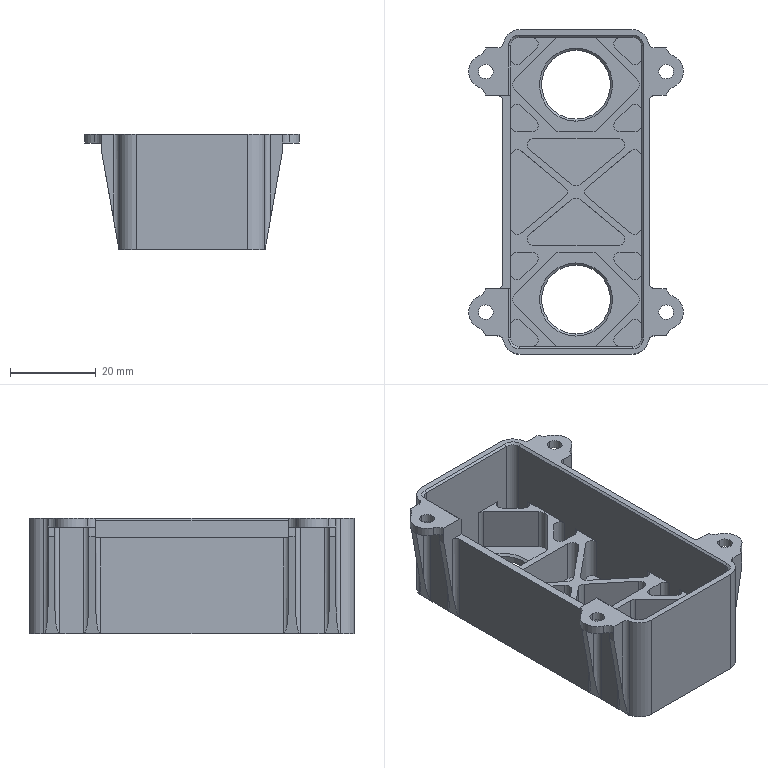NC program | NX | posted with a generic post | part box 50 x 75.58 x 26.8 mm
Lines 2647 to 3615 of 35818:
(CAVITY_MILL_COPY_COPY , TOOL : D4)
N5268 T11 M6
N5270 G54
N5272 G17 G0 G90 X-12.812 Y-30.466 S9500 M3
N5274 G43 Z30. H11
N5276 Z0.912
N5278 G94 G1 Z-0.088 F1000.
N5280 X-13.112 Y-30.639
N5282 G3 X-13.612 Y-31.505 R1.
N5284 G1 Y-33.99 F1400.
N5286 G3 X-13.2 Y-34.402 R0.412
N5288 G1 X-10.715
N5290 G3 X-9.849 Y-33.902 R1.
N5292 G1 X-9.676 Y-33.602
N5294 Z0.912
N5296 G0 X-12.413 Y-30.067 Z0.513
N5298 G1 Z-0.487 F1000.
N5300 X-12.713 Y-30.24
N5302 G3 X-13.213 Y-31.106 R1.
N5304 G1 Y-33.99 F1400.
N5306 X-13.214 Y-34.004
N5308 X-13.2 Y-34.003
N5310 X-10.316
N5312 G3 X-9.45 Y-33.503 R1.
N5314 G1 X-9.277 Y-33.203
N5316 Z0.513
N5318 G0 X-12.4 Y-30.054 Z0.114
N5320 G1 Z-0.886 F1000.
N5322 X-12.7 Y-30.227
N5324 G3 X-13.2 Y-31.093 R1.
N5326 G1 Y-33.99 F1400.
N5328 X-10.303
N5330 G3 X-9.437 Y-33.49 R1.
N5332 G1 X-9.264 Y-33.19
N5334 Z0.114
N5336 G0 X-12.4 Y-30.054 Z-0.284
N5338 G1 Z-1.284 F1000.
N5340 X-12.7 Y-30.227
N5342 G3 X-13.2 Y-31.093 R1.
N5344 G1 Y-33.99 F1400.
N5346 X-10.303
N5348 G3 X-9.437 Y-33.49 R1.
N5350 G1 X-9.264 Y-33.19
N5352 Z-0.284
N5354 G0 X-12.4 Y-30.054 Z-0.683
N5356 G1 Z-1.683 F1000.
N5358 X-12.7 Y-30.227
N5360 G3 X-13.2 Y-31.093 R1.
N5362 G1 Y-33.99 F1400.
N5364 X-10.303
N5366 G3 X-9.437 Y-33.49 R1.
N5368 G1 X-9.264 Y-33.19
N5370 Z-0.683
N5372 G0 X-12.4 Y-30.054 Z-1.082
N5374 G1 Z-2.082 F1000.
N5376 X-12.7 Y-30.227
N5378 G3 X-13.2 Y-31.093 R1.
N5380 G1 Y-33.99 F1400.
N5382 X-10.303
N5384 G3 X-9.437 Y-33.49 R1.
N5386 G1 X-9.264 Y-33.19
N5388 Z-1.082
N5390 G0 X-12.4 Y-30.054 Z-1.48
N5392 G1 Z-2.48 F1000.
N5394 X-12.7 Y-30.227
N5396 G3 X-13.2 Y-31.093 R1.
N5398 G1 Y-33.99 F1400.
N5400 X-10.303
N5402 G3 X-9.437 Y-33.49 R1.
N5404 G1 X-9.264 Y-33.19
N5406 Z-1.48
N5408 G0 X-12.4 Y-30.054 Z-1.879
N5410 G1 Z-2.879 F1000.
N5412 X-12.7 Y-30.227
N5414 G3 X-13.2 Y-31.093 R1.
N5416 G1 Y-33.99 F1400.
N5418 X-10.303
N5420 G3 X-9.437 Y-33.49 R1.
N5422 G1 X-9.264 Y-33.19
N5424 Z-1.879
N5426 G0 X-12.4 Y-30.054 Z-2.278
N5428 G1 Z-3.278 F1000.
N5430 X-12.7 Y-30.227
N5432 G3 X-13.2 Y-31.093 R1.
N5434 G1 Y-33.99 F1400.
N5436 X-10.303
N5438 G3 X-9.437 Y-33.49 R1.
N5440 G1 X-9.264 Y-33.19
N5442 Z-2.278
N5444 G0 X-12.4 Y-30.054 Z-2.676
N5446 G1 Z-3.676 F1000.
N5448 X-12.7 Y-30.227
N5450 G3 X-13.2 Y-31.093 R1.
N5452 G1 Y-33.99 F1400.
N5454 X-10.303
N5456 G3 X-9.437 Y-33.49 R1.
N5458 G1 X-9.264 Y-33.19
N5460 Z-2.676
N5462 G0 X-12.4 Y-30.054 Z-3.075
N5464 G1 Z-4.075 F1000.
N5466 X-12.7 Y-30.227
N5468 G3 X-13.2 Y-31.093 R1.
N5470 G1 Y-33.99 F1400.
N5472 X-10.303
N5474 G3 X-9.437 Y-33.49 R1.
N5476 G1 X-9.264 Y-33.19
N5478 Z-3.075
N5480 G0 X-12.4 Y-30.054 Z-3.474
N5482 G1 Z-4.474 F1000.
N5484 X-12.7 Y-30.227
N5486 G3 X-13.2 Y-31.093 R1.
N5488 G1 Y-33.99 F1400.
N5490 X-10.303
N5492 G3 X-9.437 Y-33.49 R1.
N5494 G1 X-9.264 Y-33.19
N5496 Z-3.474
N5498 G0 X-12.4 Y-30.054 Z-3.872
N5500 G1 Z-4.872 F1000.
N5502 X-12.7 Y-30.227
N5504 G3 X-13.2 Y-31.093 R1.
N5506 G1 Y-33.99 F1400.
N5508 X-10.303
N5510 G3 X-9.437 Y-33.49 R1.
N5512 G1 X-9.264 Y-33.19
N5514 Z-3.872
N5516 G0 X-12.4 Y-30.054 Z-4.271
N5518 G1 Z-5.271 F1000.
N5520 X-12.7 Y-30.227
N5522 G3 X-13.2 Y-31.093 R1.
N5524 G1 Y-33.99 F1400.
N5526 X-10.303
N5528 G3 X-9.437 Y-33.49 R1.
N5530 G1 X-9.264 Y-33.19
N5532 Z-4.271
N5534 G0 X-12.4 Y-30.054 Z-4.67
N5536 G1 Z-5.67 F1000.
N5538 X-12.7 Y-30.227
N5540 G3 X-13.2 Y-31.093 R1.
N5542 G1 Y-33.99 F1400.
N5544 X-10.303
N5546 G3 X-9.437 Y-33.49 R1.
N5548 G1 X-9.264 Y-33.19
N5550 Z-4.67
N5552 G0 X-12.4 Y-30.054 Z-5.068
N5554 G1 Z-6.068 F1000.
N5556 X-12.7 Y-30.227
N5558 G3 X-13.2 Y-31.093 R1.
N5560 G1 Y-33.99 F1400.
N5562 X-10.303
N5564 G3 X-9.437 Y-33.49 R1.
N5566 G1 X-9.264 Y-33.19
N5568 Z-5.068
N5570 G0 X-12.4 Y-30.054 Z-5.467
N5572 G1 Z-6.467 F1000.
N5574 X-12.7 Y-30.227
N5576 G3 X-13.2 Y-31.093 R1.
N5578 G1 Y-33.99 F1400.
N5580 X-10.303
N5582 G3 X-9.437 Y-33.49 R1.
N5584 G1 X-9.264 Y-33.19
N5586 Z-5.467
N5588 G0 X-12.4 Y-30.054 Z-5.866
N5590 G1 Z-6.866 F1000.
N5592 X-12.7 Y-30.227
N5594 G3 X-13.2 Y-31.093 R1.
N5596 G1 Y-33.99 F1400.
N5598 X-10.303
N5600 G3 X-9.437 Y-33.49 R1.
N5602 G1 X-9.264 Y-33.19
N5604 Z-5.866
N5606 G0 X-12.4 Y-30.054 Z-6.264
N5608 G1 Z-7.264 F1000.
N5610 X-12.7 Y-30.227
N5612 G3 X-13.2 Y-31.093 R1.
N5614 G1 Y-33.99 F1400.
N5616 X-10.303
N5618 G3 X-9.437 Y-33.49 R1.
N5620 G1 X-9.264 Y-33.19
N5622 Z-6.264
N5624 G0 X-12.4 Y-30.054 Z-6.663
N5626 G1 Z-7.663 F1000.
N5628 X-12.7 Y-30.227
N5630 G3 X-13.2 Y-31.093 R1.
N5632 G1 Y-33.99 F1400.
N5634 X-10.303
N5636 G3 X-9.437 Y-33.49 R1.
N5638 G1 X-9.264 Y-33.19
N5640 Z-6.663
N5642 G0 X-12.4 Y-30.054 Z-7.062
N5644 G1 Z-8.062 F1000.
N5646 X-12.7 Y-30.227
N5648 G3 X-13.2 Y-31.093 R1.
N5650 G1 Y-33.99 F1400.
N5652 X-10.303
N5654 G3 X-9.437 Y-33.49 R1.
N5656 G1 X-9.264 Y-33.19
N5658 Z-7.062
N5660 G0 X-12.4 Y-30.054 Z-7.461
N5662 G1 Z-8.461 F1000.
N5664 X-12.7 Y-30.227
N5666 G3 X-13.2 Y-31.093 R1.
N5668 G1 Y-33.99 F1400.
N5670 X-10.303
N5672 G3 X-9.437 Y-33.49 R1.
N5674 G1 X-9.264 Y-33.19
N5676 Z-7.461
N5678 G0 X-12.4 Y-30.054 Z-7.859
N5680 G1 Z-8.859 F1000.
N5682 X-12.7 Y-30.227
N5684 G3 X-13.2 Y-31.093 R1.
N5686 G1 Y-33.99 F1400.
N5688 X-10.303
N5690 G3 X-9.437 Y-33.49 R1.
N5692 G1 X-9.264 Y-33.19
N5694 Z-7.859
N5696 G0 X-12.4 Y-30.054 Z-8.258
N5698 G1 Z-9.258 F1000.
N5700 X-12.7 Y-30.227
N5702 G3 X-13.2 Y-31.093 R1.
N5704 G1 Y-33.99 F1400.
N5706 X-10.303
N5708 G3 X-9.437 Y-33.49 R1.
N5710 G1 X-9.264 Y-33.19
N5712 Z-8.258
N5714 G0 X-12.4 Y-30.054 Z-8.657
N5716 G1 Z-9.657 F1000.
N5718 X-12.7 Y-30.227
N5720 G3 X-13.2 Y-31.093 R1.
N5722 G1 Y-33.99 F1400.
N5724 X-10.303
N5726 G3 X-9.437 Y-33.49 R1.
N5728 G1 X-9.264 Y-33.19
N5730 Z-8.657
N5732 G0 X-12.4 Y-30.054 Z-9.055
N5734 G1 Z-10.055 F1000.
N5736 X-12.7 Y-30.227
N5738 G3 X-13.2 Y-31.093 R1.
N5740 G1 Y-33.99 F1400.
N5742 X-10.303
N5744 G3 X-9.437 Y-33.49 R1.
N5746 G1 X-9.264 Y-33.19
N5748 Z-9.055
N5750 G0 X-12.4 Y-30.054 Z-9.454
N5752 G1 Z-10.454 F1000.
N5754 X-12.7 Y-30.227
N5756 G3 X-13.2 Y-31.093 R1.
N5758 G1 Y-33.99 F1400.
N5760 X-10.303
N5762 G3 X-9.437 Y-33.49 R1.
N5764 G1 X-9.264 Y-33.19
N5766 Z-9.454
N5768 G0 X-12.4 Y-30.054 Z-9.853
N5770 G1 Z-10.853 F1000.
N5772 X-12.7 Y-30.227
N5774 G3 X-13.2 Y-31.093 R1.
N5776 G1 Y-33.99 F1400.
N5778 X-10.303
N5780 G3 X-9.437 Y-33.49 R1.
N5782 G1 X-9.264 Y-33.19
N5784 Z-9.853
N5786 G0 X-12.4 Y-30.054 Z-10.251
N5788 G1 Z-11.251 F1000.
N5790 X-12.7 Y-30.227
N5792 G3 X-13.2 Y-31.093 R1.
N5794 G1 Y-33.99 F1400.
N5796 X-10.303
N5798 G3 X-9.437 Y-33.49 R1.
N5800 G1 X-9.264 Y-33.19
N5802 Z-10.251
N5804 G0 X-12.4 Y-30.054 Z-10.65
N5806 G1 Z-11.65 F1000.
N5808 X-12.7 Y-30.227
N5810 G3 X-13.2 Y-31.093 R1.
N5812 G1 Y-33.99 F1400.
N5814 X-10.303
N5816 G3 X-9.437 Y-33.49 R1.
N5818 G1 X-9.264 Y-33.19
N5820 Z-10.65
N5822 G0 X-12.4 Y-30.054 Z-11.049
N5824 G1 Z-12.049 F1000.
N5826 X-12.7 Y-30.227
N5828 G3 X-13.2 Y-31.093 R1.
N5830 G1 Y-33.99 F1400.
N5832 X-10.303
N5834 G3 X-9.437 Y-33.49 R1.
N5836 G1 X-9.264 Y-33.19
N5838 Z-11.049
N5840 G0 X-12.4 Y-30.054 Z-11.447
N5842 G1 Z-12.447 F1000.
N5844 X-12.7 Y-30.227
N5846 G3 X-13.2 Y-31.093 R1.
N5848 G1 Y-33.99 F1400.
N5850 X-10.303
N5852 G3 X-9.437 Y-33.49 R1.
N5854 G1 X-9.264 Y-33.19
N5856 Z-11.447
N5858 G0 X-12.4 Y-30.054 Z-11.846
N5860 G1 Z-12.846 F1000.
N5862 X-12.7 Y-30.227
N5864 G3 X-13.2 Y-31.093 R1.
N5866 G1 Y-33.99 F1400.
N5868 X-10.303
N5870 G3 X-9.437 Y-33.49 R1.
N5872 G1 X-9.264 Y-33.19
N5874 Z-11.846
N5876 G0 X-12.4 Y-30.054 Z-12.245
N5878 G1 Z-13.245 F1000.
N5880 X-12.7 Y-30.227
N5882 G3 X-13.2 Y-31.093 R1.
N5884 G1 Y-33.99 F1400.
N5886 X-10.303
N5888 G3 X-9.437 Y-33.49 R1.
N5890 G1 X-9.264 Y-33.19
N5892 Z-12.245
N5894 G0 X-12.4 Y-30.054 Z-12.643
N5896 G1 Z-13.643 F1000.
N5898 X-12.7 Y-30.227
N5900 G3 X-13.2 Y-31.093 R1.
N5902 G1 Y-33.99 F1400.
N5904 X-10.303
N5906 G3 X-9.437 Y-33.49 R1.
N5908 G1 X-9.264 Y-33.19
N5910 Z-12.643
N5912 G0 X-12.4 Y-30.054 Z-13.042
N5914 G1 Z-14.042 F1000.
N5916 X-12.7 Y-30.227
N5918 G3 X-13.2 Y-31.093 R1.
N5920 G1 Y-33.99 F1400.
N5922 X-10.303
N5924 G3 X-9.437 Y-33.49 R1.
N5926 G1 X-9.264 Y-33.19
N5928 Z-13.042
N5930 G0 X-12.4 Y-30.054 Z-13.441
N5932 G1 Z-14.441 F1000.
N5934 X-12.7 Y-30.227
N5936 G3 X-13.2 Y-31.093 R1.
N5938 G1 Y-33.99 F1400.
N5940 X-10.303
N5942 G3 X-9.437 Y-33.49 R1.
N5944 G1 X-9.264 Y-33.19
N5946 Z-13.441
N5948 G0 X-13.2 Y-33.39
N5950 G1 Y-33.99 Z-13.472 F1000.
N5952 X-11.502 Z-13.561
N5954 X-13.2 Y-32.292 Z-13.687
N5956 Y-33.99 Z-13.776
N5958 X-11.502 Z-13.865
N5960 X-13.2 Y-32.292 Z-13.991
N5962 Y-33.99 Z-14.08
N5964 X-11.502 Z-14.169
N5966 X-13.2 Y-32.292 Z-14.295
N5968 Y-33.99 Z-14.384
N5970 X-11.502 Z-14.473
N5972 X-13.2 Y-32.292 Z-14.599
N5974 Y-33.99 Z-14.688
N5976 X-11.502 Z-14.777
N5978 X-12.351 Y-33.141 Z-14.839
N5980 X-13.2 Y-32.292 F1400.
N5982 Y-33.99
N5984 X-11.502
N5986 X-12.351 Y-33.141
N5988 G3 X-12.834 Y-33.012 R0.5
N5990 G1 Z-13.839
N5992 G0 X-13.2 Y-33.39
N5994 G1 Y-33.99 Z-13.871 F1000.
N5996 X-11.502 Z-13.96
N5998 X-13.2 Y-32.292 Z-14.086
N6000 Y-33.99 Z-14.175
N6002 X-11.502 Z-14.264
N6004 X-13.2 Y-32.292 Z-14.39
N6006 Y-33.99 Z-14.479
N6008 X-11.502 Z-14.568
N6010 X-13.2 Y-32.292 Z-14.693
N6012 Y-33.99 Z-14.782
N6014 X-11.502 Z-14.871
N6016 X-13.2 Y-32.292 Z-14.997
N6018 Y-33.99 Z-15.086
N6020 X-11.502 Z-15.175
N6022 X-12.351 Y-33.141 Z-15.238
N6024 X-13.2 Y-32.292 F1400.
N6026 Y-33.99
N6028 X-11.502
N6030 X-12.351 Y-33.141
N6032 G3 X-12.834 Y-33.012 R0.5
N6034 G1 Z-14.238
N6036 G0 X-13.2 Y-33.39
N6038 G1 Y-33.99 Z-14.27 F1000.
N6040 X-11.502 Z-14.359
N6042 X-13.2 Y-32.292 Z-14.484
N6044 Y-33.99 Z-14.573
N6046 X-11.502 Z-14.662
N6048 X-13.2 Y-32.292 Z-14.788
N6050 Y-33.99 Z-14.877
N6052 X-11.502 Z-14.966
N6054 X-13.2 Y-32.292 Z-15.092
N6056 Y-33.99 Z-15.181
N6058 X-11.502 Z-15.27
N6060 X-13.2 Y-32.292 Z-15.396
N6062 Y-33.99 Z-15.485
N6064 X-11.502 Z-15.574
N6066 X-12.351 Y-33.141 Z-15.637
N6068 X-13.2 Y-32.292 F1400.
N6070 Y-33.99
N6072 X-11.502
N6074 X-12.351 Y-33.141
N6076 G3 X-12.834 Y-33.012 R0.5
N6078 G1 Z-14.637
N6080 G0 X-13.2 Y-33.39
N6082 G1 Y-33.99 Z-14.668 F1000.
N6084 X-11.502 Z-14.757
N6086 X-13.2 Y-32.292 Z-14.883
N6088 Y-33.99 Z-14.972
N6090 X-11.502 Z-15.061
N6092 X-13.2 Y-32.292 Z-15.187
N6094 Y-33.99 Z-15.276
N6096 X-11.502 Z-15.365
N6098 X-13.2 Y-32.292 Z-15.491
N6100 Y-33.99 Z-15.58
N6102 X-11.502 Z-15.669
N6104 X-13.2 Y-32.292 Z-15.795
N6106 Y-33.99 Z-15.884
N6108 X-11.502 Z-15.973
N6110 X-12.351 Y-33.141 Z-16.036
N6112 X-13.2 Y-32.292 F1400.
N6114 Y-33.99
N6116 X-11.502
N6118 X-12.351 Y-33.141
N6120 G3 X-12.834 Y-33.012 R0.5
N6122 G1 Z-15.036
N6124 G0 X-13.2 Y-33.39
N6126 G1 Y-33.99 Z-15.067 F1000.
N6128 X-11.502 Z-15.156
N6130 X-13.2 Y-32.292 Z-15.282
N6132 Y-33.99 Z-15.371
N6134 X-11.502 Z-15.46
N6136 X-13.2 Y-32.292 Z-15.586
N6138 Y-33.99 Z-15.675
N6140 X-11.502 Z-15.764
N6142 X-13.2 Y-32.292 Z-15.889
N6144 Y-33.99 Z-15.978
N6146 X-11.502 Z-16.067
N6148 X-13.2 Y-32.292 Z-16.193
N6150 Y-33.99 Z-16.282
N6152 X-11.502 Z-16.371
N6154 X-12.351 Y-33.141 Z-16.434
N6156 X-13.2 Y-32.292 F1400.
N6158 Y-33.99
N6160 X-11.502
N6162 X-12.351 Y-33.141
N6164 G3 X-12.834 Y-33.012 R0.5
N6166 G1 Z-15.434
N6168 G0 X-13.2 Y-33.39
N6170 G1 Y-33.99 Z-15.466 F1000.
N6172 X-11.502 Z-15.555
N6174 X-13.2 Y-32.292 Z-15.68
N6176 Y-33.99 Z-15.769
N6178 X-11.502 Z-15.858
N6180 X-13.2 Y-32.292 Z-15.984
N6182 Y-33.99 Z-16.073
N6184 X-11.502 Z-16.162
N6186 X-13.2 Y-32.292 Z-16.288
N6188 Y-33.99 Z-16.377
N6190 X-11.502 Z-16.466
N6192 X-13.2 Y-32.292 Z-16.592
N6194 Y-33.99 Z-16.681
N6196 X-11.502 Z-16.77
N6198 X-12.351 Y-33.141 Z-16.833
N6200 X-13.2 Y-32.292 F1400.
N6202 Y-33.99
N6204 X-11.502
N6206 X-12.351 Y-33.141
N6208 G3 X-12.834 Y-33.012 R0.5
N6210 G1 Z-15.833
N6212 G0 X-13.2 Y-33.39
N6214 G1 Y-33.99 Z-15.864 F1000.
N6216 X-11.502 Z-15.953
N6218 X-13.2 Y-32.292 Z-16.079
N6220 Y-33.99 Z-16.168
N6222 X-11.502 Z-16.257
N6224 X-13.2 Y-32.292 Z-16.383
N6226 Y-33.99 Z-16.472
N6228 X-11.502 Z-16.561
N6230 X-13.2 Y-32.292 Z-16.687
N6232 Y-33.99 Z-16.776
N6234 X-11.502 Z-16.865
N6236 X-13.2 Y-32.292 Z-16.991
N6238 Y-33.99 Z-17.08
N6240 X-11.502 Z-17.169
N6242 X-12.351 Y-33.141 Z-17.232
N6244 X-13.2 Y-32.292 F1400.
N6246 Y-33.99
N6248 X-11.502
N6250 X-12.351 Y-33.141
N6252 G3 X-12.834 Y-33.012 R0.5
N6254 G1 Z-16.232
N6256 G0 X-13.2 Y-33.39
N6258 G1 Y-33.99 Z-16.263 F1000.
N6260 X-11.502 Z-16.352
N6262 X-13.2 Y-32.292 Z-16.478
N6264 Y-33.99 Z-16.567
N6266 X-11.502 Z-16.656
N6268 X-13.2 Y-32.292 Z-16.782
N6270 Y-33.99 Z-16.871
N6272 X-11.502 Z-16.96
N6274 X-13.2 Y-32.292 Z-17.086
N6276 Y-33.99 Z-17.175
N6278 X-11.502 Z-17.264
N6280 X-13.2 Y-32.292 Z-17.389
N6282 Y-33.99 Z-17.478
N6284 X-11.502 Z-17.567
N6286 X-12.351 Y-33.141 Z-17.63
N6288 X-13.2 Y-32.292 F1400.
N6290 Y-33.99
N6292 X-11.502
N6294 X-12.351 Y-33.141
N6296 G3 X-12.834 Y-33.012 R0.5
N6298 G1 Z-16.63
N6300 G0 X-13.2 Y-33.39
N6302 G1 Y-33.99 Z-16.662 F1000.
N6304 X-11.502 Z-16.751
N6306 X-13.2 Y-32.292 Z-16.877
N6308 Y-33.99 Z-16.966
N6310 X-11.502 Z-17.055
N6312 X-13.2 Y-32.292 Z-17.18
N6314 Y-33.99 Z-17.269
N6316 X-11.502 Z-17.358
N6318 X-13.2 Y-32.292 Z-17.484
N6320 Y-33.99 Z-17.573
N6322 X-11.502 Z-17.662
N6324 X-13.2 Y-32.292 Z-17.788
N6326 Y-33.99 Z-17.877
N6328 X-11.502 Z-17.966
N6330 X-12.351 Y-33.141 Z-18.029
N6332 X-13.2 Y-32.292 F1400.
N6334 Y-33.99
N6336 X-11.502
N6338 X-12.351 Y-33.141
N6340 G3 X-12.834 Y-33.012 R0.5
N6342 G1 Z-17.029
N6344 G0 X-13.2 Y-33.39
N6346 G1 Y-33.99 Z-17.06 F1000.
N6348 X-11.502 Z-17.149
N6350 X-13.2 Y-32.292 Z-17.275
N6352 Y-33.99 Z-17.364
N6354 X-11.502 Z-17.453
N6356 X-13.2 Y-32.292 Z-17.579
N6358 Y-33.99 Z-17.668
N6360 X-11.502 Z-17.757
N6362 X-13.2 Y-32.292 Z-17.883
N6364 Y-33.99 Z-17.972
N6366 X-11.502 Z-18.061
N6368 X-13.2 Y-32.292 Z-18.187
N6370 Y-33.99 Z-18.276
N6372 X-11.502 Z-18.365
N6374 X-12.351 Y-33.141 Z-18.428
N6376 X-13.2 Y-32.292 F1400.
N6378 Y-33.99
N6380 X-11.502
N6382 X-12.351 Y-33.141
N6384 G3 X-12.834 Y-33.012 R0.5
N6386 G1 Z-17.428
N6388 G0 X-13.2 Y-33.39
N6390 G1 Y-33.99 Z-17.459 F1000.
N6392 X-11.502 Z-17.548
N6394 X-13.2 Y-32.292 Z-17.674
N6396 Y-33.99 Z-17.763
N6398 X-11.502 Z-17.852
N6400 X-13.2 Y-32.292 Z-17.978
N6402 Y-33.99 Z-18.067
N6404 X-11.502 Z-18.156
N6406 X-13.2 Y-32.292 Z-18.282
N6408 Y-33.99 Z-18.371
N6410 X-11.502 Z-18.46
N6412 X-13.2 Y-32.292 Z-18.585
N6414 Y-33.99 Z-18.674
N6416 X-11.502 Z-18.763
N6418 X-12.351 Y-33.141 Z-18.826
N6420 X-13.2 Y-32.292 F1400.
N6422 Y-33.99
N6424 X-11.502
N6426 X-12.351 Y-33.141
N6428 G3 X-12.834 Y-33.012 R0.5
N6430 G1 Z-17.826
N6432 G0 X-13.2 Y-33.39
N6434 G1 Y-33.99 Z-17.858 F1000.
N6436 X-11.502 Z-17.947
N6438 X-13.2 Y-32.292 Z-18.073
N6440 Y-33.99 Z-18.162
N6442 X-11.502 Z-18.251
N6444 X-13.2 Y-32.292 Z-18.376
N6446 Y-33.99 Z-18.465
N6448 X-11.502 Z-18.554
N6450 X-13.2 Y-32.292 Z-18.68
N6452 Y-33.99 Z-18.769
N6454 X-11.502 Z-18.858
N6456 X-13.2 Y-32.292 Z-18.984
N6458 Y-33.99 Z-19.073
N6460 X-11.502 Z-19.162
N6462 X-12.351 Y-33.141 Z-19.225
N6464 X-13.2 Y-32.292 F1400.
N6466 Y-33.99
N6468 X-11.502
N6470 X-12.351 Y-33.141
N6472 G3 X-12.834 Y-33.012 R0.5
N6474 G1 Z-18.225
N6476 G0 X-13.2 Y-33.39
N6478 G1 Y-33.99 Z-18.256 F1000.
N6480 X-11.502 Z-18.345
N6482 X-13.2 Y-32.292 Z-18.471
N6484 Y-33.99 Z-18.56
N6486 X-11.502 Z-18.649
N6488 X-13.2 Y-32.292 Z-18.775
N6490 Y-33.99 Z-18.864
N6492 X-11.502 Z-18.953
N6494 X-13.2 Y-32.292 Z-19.079
N6496 Y-33.99 Z-19.168
N6498 X-11.502 Z-19.257
N6500 X-13.2 Y-32.292 Z-19.383
N6502 Y-33.99 Z-19.472
N6504 X-11.502 Z-19.561
N6506 X-12.351 Y-33.141 Z-19.624
N6508 X-13.2 Y-32.292 F1400.
N6510 Y-33.99
N6512 X-11.502
N6514 X-12.351 Y-33.141
N6516 G3 X-12.834 Y-33.012 R0.5
N6518 G1 Z-18.624
N6520 G0 X-13.2 Y-33.39
N6522 G1 Y-33.99 Z-18.655 F1000.
N6524 X-11.502 Z-18.744
N6526 X-13.2 Y-32.292 Z-18.87
N6528 Y-33.99 Z-18.959
N6530 X-11.502 Z-19.048
N6532 X-13.2 Y-32.292 Z-19.174
N6534 Y-33.99 Z-19.263
N6536 X-11.502 Z-19.352
N6538 X-13.2 Y-32.292 Z-19.478
N6540 Y-33.99 Z-19.567
N6542 X-11.502 Z-19.656
N6544 X-13.2 Y-32.292 Z-19.781
N6546 Y-33.99 Z-19.87
N6548 X-11.502 Z-19.959
N6550 X-12.351 Y-33.141 Z-20.022
N6552 X-13.2 Y-32.292 F1400.
N6554 Y-33.99
N6556 X-11.502
N6558 X-12.351 Y-33.141
N6560 G3 X-12.834 Y-33.012 R0.5
N6562 G1 Z-19.022
N6564 G0 X-13.2 Y-33.39
N6566 G1 Y-33.99 Z-19.054 F1000.
N6568 X-11.502 Z-19.143
N6570 X-13.2 Y-32.292 Z-19.269
N6572 Y-33.99 Z-19.358
N6574 X-11.502 Z-19.447
N6576 X-13.2 Y-32.292 Z-19.572
N6578 Y-33.99 Z-19.661
N6580 X-11.502 Z-19.75
N6582 X-13.2 Y-32.292 Z-19.876
N6584 Y-33.99 Z-19.965
N6586 X-11.502 Z-20.054
N6588 X-13.2 Y-32.292 Z-20.18
N6590 Y-33.99 Z-20.269
N6592 X-11.502 Z-20.358
N6594 X-12.351 Y-33.141 Z-20.421
N6596 X-13.2 Y-32.292 F1400.
N6598 Y-33.99
N6600 X-11.502
N6602 X-12.351 Y-33.141
N6604 G3 X-12.834 Y-33.012 R0.5
N6606 G1 Z-19.421
N6608 G0 X-13.2 Y-33.39
N6610 G1 Y-33.99 Z-19.452 F1000.
N6612 X-11.502 Z-19.541
N6614 X-13.2 Y-32.292 Z-19.667
N6616 Y-33.99 Z-19.756
N6618 X-11.502 Z-19.845
N6620 X-13.2 Y-32.292 Z-19.971
N6622 Y-33.99 Z-20.06
N6624 X-11.502 Z-20.149
N6626 X-13.2 Y-32.292 Z-20.275
N6628 Y-33.99 Z-20.364
N6630 X-11.502 Z-20.453
N6632 X-13.2 Y-32.292 Z-20.579
N6634 Y-33.99 Z-20.668
N6636 X-11.502 Z-20.757
N6638 X-12.351 Y-33.141 Z-20.82
N6640 X-13.2 Y-32.292 F1400.
N6642 Y-33.99
N6644 X-11.502
N6646 X-12.351 Y-33.141
N6648 G3 X-12.834 Y-33.012 R0.5
N6650 G1 Z-19.82
N6652 G0 X-13.2 Y-33.39
N6654 G1 Y-33.99 Z-19.851 F1000.
N6656 X-11.502 Z-19.94
N6658 X-13.2 Y-32.292 Z-20.066
N6660 Y-33.99 Z-20.155
N6662 X-11.502 Z-20.244
N6664 X-13.2 Y-32.292 Z-20.37
N6666 Y-33.99 Z-20.459
N6668 X-11.502 Z-20.548
N6670 X-13.2 Y-32.292 Z-20.674
N6672 Y-33.99 Z-20.763
N6674 X-11.502 Z-20.852
N6676 X-13.2 Y-32.292 Z-20.978
N6678 Y-33.99 Z-21.067
N6680 X-11.502 Z-21.155
N6682 X-12.351 Y-33.141 Z-21.218
N6684 X-13.2 Y-32.292 F1400.
N6686 Y-33.99
N6688 X-11.502
N6690 X-12.351 Y-33.141
N6692 G3 X-12.834 Y-33.012 R0.5
N6694 G1 Z-20.218
N6696 G0 X-13.2 Y-33.39
N6698 G1 Y-33.99 Z-20.25 F1000.
N6700 X-11.502 Z-20.339
N6702 X-13.2 Y-32.292 Z-20.465
N6704 Y-33.99 Z-20.554
N6706 X-11.502 Z-20.643
N6708 X-13.2 Y-32.292 Z-20.769
N6710 Y-33.99 Z-20.858
N6712 X-11.502 Z-20.947
N6714 X-13.2 Y-32.292 Z-21.072
N6716 Y-33.99 Z-21.161
N6718 X-11.502 Z-21.25
N6720 X-13.2 Y-32.292 Z-21.376
N6722 Y-33.99 Z-21.465
N6724 X-11.502 Z-21.554
N6726 X-12.351 Y-33.141 Z-21.617
N6728 X-13.2 Y-32.292 F1400.
N6730 Y-33.99
N6732 X-11.502
N6734 X-12.351 Y-33.141
N6736 G3 X-12.834 Y-33.012 R0.5
N6738 G1 Z-20.617
N6740 G0 X-13.2 Y-33.39
N6742 G1 Y-33.99 Z-20.649 F1000.
N6744 X-11.502 Z-20.738
N6746 X-13.2 Y-32.292 Z-20.863
N6748 Y-33.99 Z-20.952
N6750 X-11.502 Z-21.041
N6752 X-13.2 Y-32.292 Z-21.167
N6754 Y-33.99 Z-21.256
N6756 X-11.502 Z-21.345
N6758 X-13.2 Y-32.292 Z-21.471
N6760 Y-33.99 Z-21.56
N6762 X-11.502 Z-21.649
N6764 X-13.2 Y-32.292 Z-21.775
N6766 Y-33.99 Z-21.864
N6768 X-11.502 Z-21.953
N6770 X-12.351 Y-33.141 Z-22.016
N6772 X-13.2 Y-32.292 F1400.
N6774 Y-33.99
N6776 X-11.502
N6778 X-12.351 Y-33.141
N6780 G3 X-12.834 Y-33.012 R0.5
N6782 G1 Z-21.016
N6784 G0 X-13.2 Y-33.39
N6786 G1 Y-33.99 Z-21.047 F1000.
N6788 X-11.502 Z-21.136
N6790 X-13.2 Y-32.292 Z-21.262
N6792 Y-33.99 Z-21.351
N6794 X-11.502 Z-21.44
N6796 X-13.2 Y-32.292 Z-21.566
N6798 Y-33.99 Z-21.655
N6800 X-11.502 Z-21.744
N6802 X-13.2 Y-32.292 Z-21.87
N6804 Y-33.99 Z-21.959
N6806 X-11.502 Z-22.048
N6808 X-13.2 Y-32.292 Z-22.174
N6810 Y-33.99 Z-22.263
N6812 X-11.502 Z-22.352
N6814 X-12.351 Y-33.141 Z-22.414
N6816 X-13.2 Y-32.292 F1400.
N6818 Y-33.99
N6820 X-11.502
N6822 X-12.351 Y-33.141
N6824 G3 X-12.834 Y-33.012 R0.5
N6826 G1 Z-21.414
N6828 G0 X-13.2 Y-33.39
N6830 G1 Y-33.99 Z-21.446 F1000.
N6832 X-11.502 Z-21.535
N6834 X-13.2 Y-32.292 Z-21.661
N6836 Y-33.99 Z-21.75
N6838 X-11.502 Z-21.839
N6840 X-13.2 Y-32.292 Z-21.965
N6842 Y-33.99 Z-22.054
N6844 X-11.502 Z-22.143
N6846 X-13.2 Y-32.292 Z-22.268
N6848 Y-33.99 Z-22.357
N6850 X-11.502 Z-22.446
N6852 X-13.2 Y-32.292 Z-22.572
N6854 Y-33.99 Z-22.661
N6856 X-11.502 Z-22.75
N6858 X-12.351 Y-33.141 Z-22.813
N6860 X-13.2 Y-32.292 F1400.
N6862 Y-33.99
N6864 X-11.502
N6866 X-12.351 Y-33.141
N6868 G3 X-12.834 Y-33.012 R0.5
N6870 G1 Z-21.813
N6872 G0 X-13.2 Y-33.39
N6874 G1 Y-33.99 Z-21.845 F1000.
N6876 X-11.502 Z-21.934
N6878 X-13.2 Y-32.292 Z-22.059
N6880 Y-33.99 Z-22.148
N6882 X-11.502 Z-22.237
N6884 X-13.2 Y-32.292 Z-22.363
N6886 Y-33.99 Z-22.452
N6888 X-11.502 Z-22.541
N6890 X-13.2 Y-32.292 Z-22.667
N6892 Y-33.99 Z-22.756
N6894 X-11.502 Z-22.845
N6896 X-13.2 Y-32.292 Z-22.971
N6898 Y-33.99 Z-23.06
N6900 X-11.502 Z-23.149
N6902 X-12.351 Y-33.141 Z-23.212
N6904 X-13.2 Y-32.292 F1400.
N6906 Y-33.99
N6908 X-11.502
N6910 X-12.351 Y-33.141
N6912 G3 X-12.834 Y-33.012 R0.5
N6914 G1 Z-22.212
N6916 G0 X-13.2 Y-33.39
N6918 G1 Y-33.99 Z-22.243 F1000.
N6920 X-11.502 Z-22.332
N6922 X-13.2 Y-32.292 Z-22.458
N6924 Y-33.99 Z-22.547
N6926 X-11.502 Z-22.636
N6928 X-13.2 Y-32.292 Z-22.762
N6930 Y-33.99 Z-22.851
N6932 X-11.502 Z-22.94
N6934 X-13.2 Y-32.292 Z-23.066
N6936 Y-33.99 Z-23.155
N6938 X-11.502 Z-23.244
N6940 X-13.2 Y-32.292 Z-23.37
N6942 Y-33.99 Z-23.459
N6944 X-11.502 Z-23.548
N6946 X-12.351 Y-33.141 Z-23.611
N6948 X-13.2 Y-32.292 F1400.
N6950 Y-33.99
N6952 X-11.502
N6954 X-12.351 Y-33.141
N6956 G3 X-12.834 Y-33.012 R0.5
N6958 G1 Z-22.611
N6960 G0 X-13.2 Y-33.39
N6962 G1 Y-33.99 Z-22.642 F1000.
N6964 X-11.502 Z-22.731
N6966 X-13.2 Y-32.292 Z-22.857
N6968 Y-33.99 Z-22.946
N6970 X-11.502 Z-23.035
N6972 X-13.2 Y-32.292 Z-23.161
N6974 Y-33.99 Z-23.25
N6976 X-11.502 Z-23.339
N6978 X-13.2 Y-32.292 Z-23.464
N6980 Y-33.99 Z-23.553
N6982 X-11.502 Z-23.642
N6984 X-13.2 Y-32.292 Z-23.768
N6986 Y-33.99 Z-23.857
N6988 X-11.502 Z-23.946
N6990 X-12.351 Y-33.141 Z-24.009
N6992 X-13.2 Y-32.292 F1400.
N6994 Y-33.99
N6996 X-11.502
N6998 X-12.351 Y-33.141
N7000 G3 X-12.834 Y-33.012 R0.5
N7002 G1 Z-23.009
N7004 G0 X-13.2 Y-33.39
N7006 G1 Y-33.99 Z-23.041 F1000.
N7008 X-11.502 Z-23.13
N7010 X-13.2 Y-32.292 Z-23.255
N7012 Y-33.99 Z-23.344
N7014 X-11.502 Z-23.433
N7016 X-13.2 Y-32.292 Z-23.559
N7018 Y-33.99 Z-23.648
N7020 X-11.502 Z-23.737
N7022 X-13.2 Y-32.292 Z-23.863
N7024 Y-33.99 Z-23.952
N7026 X-11.502 Z-24.041
N7028 X-13.2 Y-32.292 Z-24.167
N7030 Y-33.99 Z-24.256
N7032 X-11.502 Z-24.345
N7034 X-12.351 Y-33.141 Z-24.408
N7036 X-13.2 Y-32.292 F1400.
N7038 Y-33.99
N7040 X-11.502
N7042 X-12.351 Y-33.141
N7044 G3 X-12.834 Y-33.012 R0.5
N7046 G1 Z-23.408
N7048 G0 X-13.2 Y-33.39
N7050 G1 Y-33.99 Z-23.439 F1000.
N7052 X-11.502 Z-23.528
N7054 X-13.2 Y-32.292 Z-23.654
N7056 Y-33.99 Z-23.743
N7058 X-11.502 Z-23.832
N7060 X-13.2 Y-32.292 Z-23.958
N7062 Y-33.99 Z-24.047
N7064 X-11.502 Z-24.136
N7066 X-13.2 Y-32.292 Z-24.262
N7068 Y-33.99 Z-24.351
N7070 X-11.502 Z-24.44
N7072 X-13.2 Y-32.292 Z-24.566
N7074 Y-33.99 Z-24.655
N7076 X-11.502 Z-24.744
N7078 X-12.351 Y-33.141 Z-24.807
N7080 X-13.2 Y-32.292 F1400.
N7082 Y-33.99
N7084 X-11.502
N7086 X-12.351 Y-33.141
N7088 G3 X-12.834 Y-33.012 R0.5
N7090 G1 Z-23.807
N7092 G0 Z30.
N7094 X-4.699 Y-31.884
N7096 Z-13.839
N7098 G1 Z-14.839 F1000.
N7100 X-4.788 Y-32.218
N7102 G3 X-4.53 Y-33.184 R1.
N7104 G1 X-3.724 Y-33.99 F1400.
N7106 X-2.584
N7108 G3 X-1.718 Y-33.49 R1.
N7110 G1 X-1.545 Y-33.19
N7112 Z-13.839
N7114 G0 X-4.699 Y-31.884 Z-14.238
N7116 G1 Z-15.238 F1000.
N7118 X-4.788 Y-32.218
N7120 G3 X-4.53 Y-33.184 R1.
N7122 G1 X-3.724 Y-33.99 F1400.
N7124 X-2.584
N7126 G3 X-1.718 Y-33.49 R1.
N7128 G1 X-1.545 Y-33.19
N7130 Z-14.238
N7132 G0 X-4.699 Y-31.884 Z-14.637
N7134 G1 Z-15.637 F1000.
N7136 X-4.788 Y-32.218
N7138 G3 X-4.53 Y-33.184 R1.
N7140 G1 X-3.724 Y-33.99 F1400.
N7142 X-2.584
N7144 G3 X-1.718 Y-33.49 R1.
N7146 G1 X-1.545 Y-33.19
N7148 Z-14.637
N7150 G0 X-4.699 Y-31.884 Z-15.036
N7152 G1 Z-16.036 F1000.
N7154 X-4.788 Y-32.218
N7156 G3 X-4.53 Y-33.184 R1.
N7158 G1 X-3.724 Y-33.99 F1400.
N7160 X-2.584
N7162 G3 X-1.718 Y-33.49 R1.
N7164 G1 X-1.545 Y-33.19
N7166 Z-15.036
N7168 G0 X-4.699 Y-31.884 Z-15.434
N7170 G1 Z-16.434 F1000.
N7172 X-4.788 Y-32.218
N7174 G3 X-4.53 Y-33.184 R1.
N7176 G1 X-3.724 Y-33.99 F1400.
N7178 X-2.584
N7180 G3 X-1.718 Y-33.49 R1.
N7182 G1 X-1.545 Y-33.19
N7184 Z-15.434
N7186 G0 X-4.699 Y-31.884 Z-15.833
N7188 G1 Z-16.833 F1000.
N7190 X-4.788 Y-32.218
N7192 G3 X-4.53 Y-33.184 R1.
N7194 G1 X-3.724 Y-33.99 F1400.
N7196 X-2.584
N7198 G3 X-1.718 Y-33.49 R1.